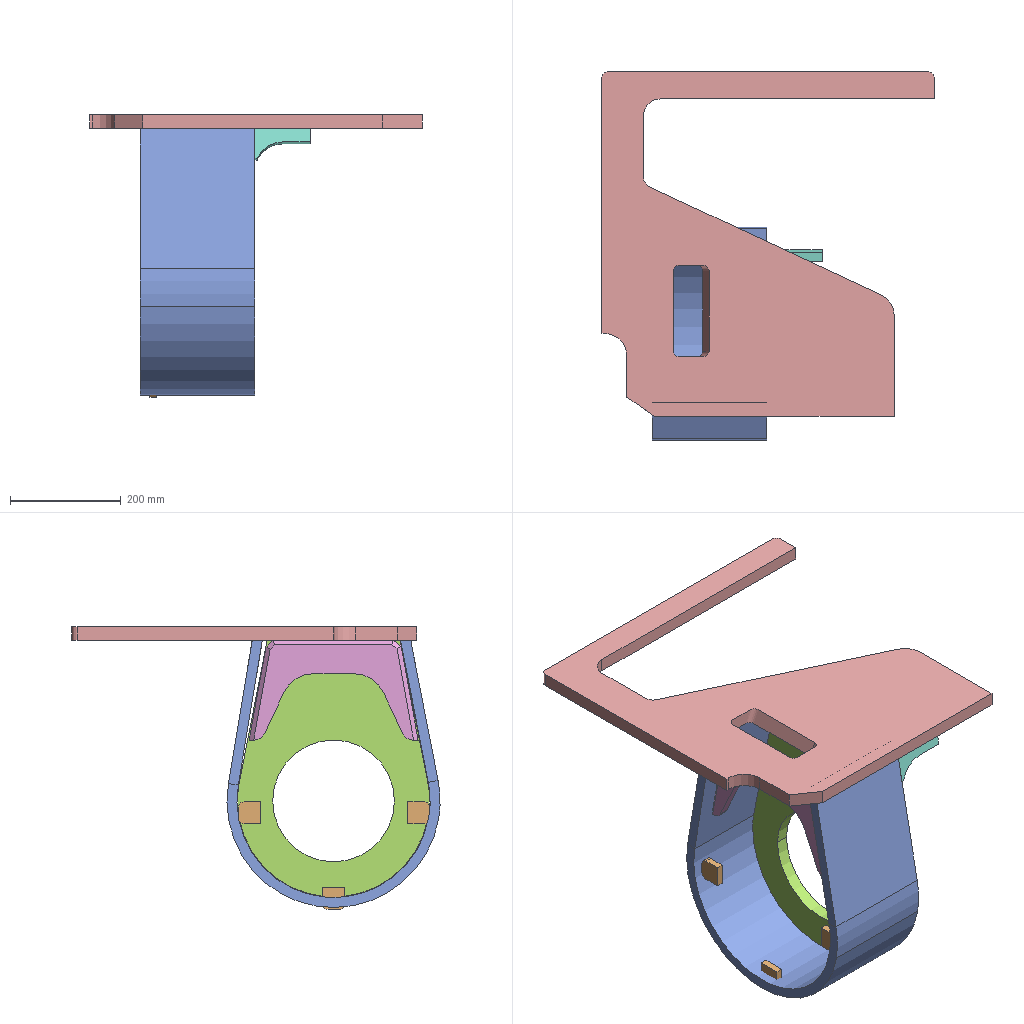Assembly | SolidWorks | 6 different items | 9 placed | box 600 x 665 x 511 mm
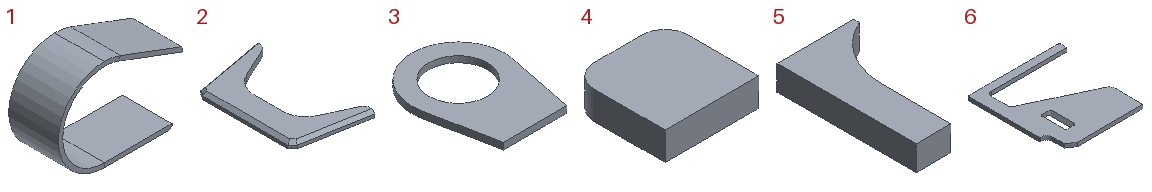Parts list (item | quantity | size | volume | features):
1 | x1 | 521.895 x 207.5 x 385 mm | 4494865 mm3 | features Chamfer 1, FlatPattern 1, SM3dBend 1, SMBaseFlange 1, SheetMetal 1
2 | x1 | 180 x 305.1 x 16 mm | 379502 mm3 | features Chamfer 2, Extrusion 1
3 | x1 | 347 x 463.5 x 25 mm | 2362679 mm3 | features Extrusion 1, ICE 1
4 | x3 | 40 x 40 x 12 mm | 18685 mm3 | features Extrusion 1
5 | x2 | 55 x 100 x 18 mm | 54165 mm3 | features Extrusion 1
6 | x1 | 600 x 622.5 x 25 mm | 4943914 mm3 | features BlendCut 1, Extrusion 1
Mates (type | each side: item.copy, entity, surface, feature):
DistanceDim | 1.1 face plane Base-Flange1 | 6.1 face plane Boss-Extrude1
Coincident | 6.1 face plane Boss-Extrude1 | 3.1 face plane Boss-Extrude1
DistanceDim | 3.1 face plane Boss-Extrude1 | 6.1 face plane Boss-Extrude1
DistanceDim | 3.1 edge | 6.1 face plane Boss-Extrude1
Concentric | 1.1 face cylinder Sketch Bend1 | 3.1 face cylinder Boss-Extrude1
Parallel | 1.1 face plane Sketched Bend1 | 3.1 face plane Boss-Extrude1
Coincident | 6.1 face plane Boss-Extrude1 | 2.1 face plane Boss-Extrude1
DistanceDim | 2.1 face plane Boss-Extrude1 | 1.1 face plane Base-Flange1
DistanceDim | 1.1 face plane Sketched Bend1 | 2.1 edge
Coincident | 1.1 face plane Base-Flange1 | 5.1 face plane Boss-Extrude1
Coincident | 1.1 face plane Sketched Bend1 | 5.1 face plane Boss-Extrude1
Coincident | 6.1 face plane Boss-Extrude1 | 5.1 edge
Coincident | 1.1 face plane Base-Flange1 | 5.2 face plane Boss-Extrude1
Coincident | 1.1 face plane Base-Flange1 | 5.2 edge
Coincident | 6.1 face plane Boss-Extrude1 | 5.2 edge
Coincident | 2.1 face plane Boss-Extrude1 | 4.1 face plane Boss-Extrude1
Coincident | 2.1 face plane Boss-Extrude1 | 4.2 face plane Boss-Extrude1
Coincident | 2.1 face plane Boss-Extrude1 | 4.3 face plane Boss-Extrude1
DistanceDim | 6.1 face plane Boss-Extrude1 | 4.3 face plane Boss-Extrude1 | 2 times
DistanceDim | 4.1 face plane Boss-Extrude1 | 6.1 face plane Boss-Extrude1
Coincident | 1.1 face cylinder Sketch Bend1 | 4.1 edge
DistanceDim | 4.2 face plane Boss-Extrude1 | 6.1 face plane Boss-Extrude1
Coincident | 1.1 face cylinder Sketch Bend1 | 4.2 edge